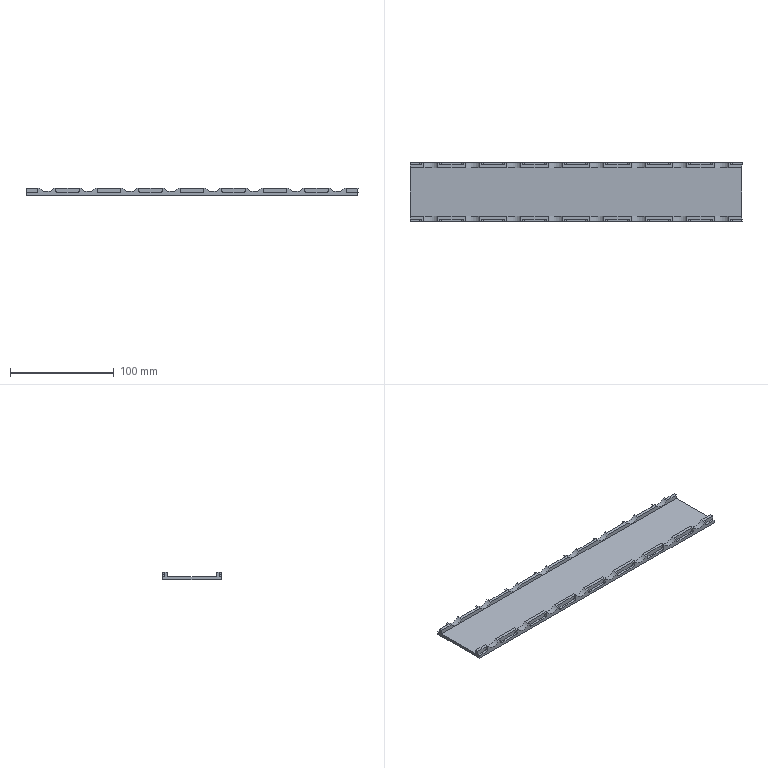NC program | Mastercam | posted with a generic post
Lines 1 to 1817 of 9376, first 1669 of 1817 lines:
%
:0001()
(MATERIAL - ALUMINUM MM - 2024)
(T1|8  RC |H1|D1|WEAR COMP|TOOL DIA. - 8.|XY STOCK TO LEAVE - .15|Z STOCK TO LEAVE - .5)
(T2|8 FI |H2)
(T3|4 RC |H3|D3|WEAR COMP|TOOL DIA. - 4.|XY STOCK TO LEAVE - .1|Z STOCK TO LEAVE - .1)
(T4|4 FI |H4|D4|WEAR COMP|TOOL DIA. - 4.)
(T5|2 BM/BNOS |H5)
N100 G21
N102 G0 G17 G40 G80 G90 G94 G98
N104 G0 G28 G91 Z0.
N106 G0 G28 X0. Y0.
(8  RC |TOOL - 1|DIA. OFF. - 1|LEN. - 1|TOOL DIA. - 8.)
N108 T1 M6
N110 G0 G54 G90 X172.55 Y.4 C0. B0. S6500 M3
N112 G43 H1 Z50.
N114 Z8.2
N116 G1 Z7.2 F2000.
N118 G41 D1 X164.55
N120 G3 X164.15 Y0. J-.4
N122 G1 Y-28.3 Z7.182
N124 X164.114 Y-28.842
N126 X164.009 Y-29.374 Z7.181
N128 X163.834 Y-29.888
N130 X163.594 Y-30.375
N132 X163.292 Y-30.826 Z7.18
N134 X162.934 Y-31.234
N136 X162.526 Y-31.592
N138 X162.075 Y-31.894 Z7.179
N140 X161.588 Y-32.134
N142 X161.074 Y-32.309
N144 X160.542 Y-32.414 Z7.178
N146 X160. Y-32.45
N148 X-160. Z6.972
N150 X-160.542 Y-32.414
N152 X-161.074 Y-32.309 Z6.971
N154 X-161.588 Y-32.134
N156 X-162.075 Y-31.894
N158 X-162.526 Y-31.592 Z6.97
N160 X-162.934 Y-31.234
N162 X-163.292 Y-30.826
N164 X-163.594 Y-30.375 Z6.969
N166 X-163.834 Y-29.888
N168 X-164.009 Y-29.374
N170 X-164.114 Y-28.842 Z6.968
N172 X-164.15 Y-28.3
N174 Y28.3 Z6.932
N176 X-164.114 Y28.842
N178 X-164.009 Y29.374 Z6.931
N180 X-163.834 Y29.888
N182 X-163.594 Y30.375
N184 X-163.292 Y30.826 Z6.93
N186 X-162.934 Y31.234
N188 X-162.526 Y31.592
N190 X-162.075 Y31.894 Z6.929
N192 X-161.588 Y32.134
N194 X-161.074 Y32.309
N196 X-160.542 Y32.414 Z6.928
N198 X-160. Y32.45
N200 X160. Z6.722
N202 X160.542 Y32.414
N204 X161.074 Y32.309 Z6.721
N206 X161.588 Y32.134
N208 X162.075 Y31.894
N210 X162.526 Y31.592 Z6.72
N212 X162.934 Y31.234
N214 X163.292 Y30.826
N216 X163.594 Y30.375 Z6.719
N218 X163.834 Y29.888
N220 X164.009 Y29.374
N222 X164.114 Y28.842 Z6.718
N224 X164.15 Y28.3
N226 Y0. Z6.7
N228 Y-28.3 Z6.682
N230 X164.114 Y-28.842
N232 X164.009 Y-29.374 Z6.681
N234 X163.834 Y-29.888
N236 X163.594 Y-30.375
N238 X163.292 Y-30.826 Z6.68
N240 X162.934 Y-31.234
N242 X162.526 Y-31.592
N244 X162.075 Y-31.894 Z6.679
N246 X161.588 Y-32.134
N248 X161.074 Y-32.309
N250 X160.542 Y-32.414 Z6.678
N252 X160. Y-32.45
N254 X-160. Z6.472
N256 X-160.542 Y-32.414
N258 X-161.074 Y-32.309 Z6.471
N260 X-161.588 Y-32.134
N262 X-162.075 Y-31.894
N264 X-162.526 Y-31.592 Z6.47
N266 X-162.934 Y-31.234
N268 X-163.292 Y-30.826
N270 X-163.594 Y-30.375 Z6.469
N272 X-163.834 Y-29.888
N274 X-164.009 Y-29.374
N276 X-164.114 Y-28.842 Z6.468
N278 X-164.15 Y-28.3
N280 Y28.3 Z6.432
N282 X-164.114 Y28.842
N284 X-164.009 Y29.374 Z6.431
N286 X-163.834 Y29.888
N288 X-163.594 Y30.375
N290 X-163.292 Y30.826 Z6.43
N292 X-162.934 Y31.234
N294 X-162.526 Y31.592
N296 X-162.075 Y31.894 Z6.429
N298 X-161.588 Y32.134
N300 X-161.074 Y32.309
N302 X-160.542 Y32.414 Z6.428
N304 X-160. Y32.45
N306 X160. Z6.222
N308 X160.542 Y32.414
N310 X161.074 Y32.309 Z6.221
N312 X161.588 Y32.134
N314 X162.075 Y31.894
N316 X162.526 Y31.592 Z6.22
N318 X162.934 Y31.234
N320 X163.292 Y30.826
N322 X163.594 Y30.375 Z6.219
N324 X163.834 Y29.888
N326 X164.009 Y29.374
N328 X164.114 Y28.842 Z6.218
N330 X164.15 Y28.3
N332 Y0. Z6.2
N334 Y-28.3 Z6.182
N336 X164.114 Y-28.842
N338 X164.009 Y-29.374 Z6.181
N340 X163.834 Y-29.888
N342 X163.594 Y-30.375
N344 X163.292 Y-30.826 Z6.18
N346 X162.934 Y-31.234
N348 X162.526 Y-31.592
N350 X162.075 Y-31.894 Z6.179
N352 X161.588 Y-32.134
N354 X161.074 Y-32.309
N356 X160.542 Y-32.414 Z6.178
N358 X160. Y-32.45
N360 X-160. Z5.972
N362 X-160.542 Y-32.414
N364 X-161.074 Y-32.309 Z5.971
N366 X-161.588 Y-32.134
N368 X-162.075 Y-31.894
N370 X-162.526 Y-31.592 Z5.97
N372 X-162.934 Y-31.234
N374 X-163.292 Y-30.826
N376 X-163.594 Y-30.375 Z5.969
N378 X-163.834 Y-29.888
N380 X-164.009 Y-29.374
N382 X-164.114 Y-28.842 Z5.968
N384 X-164.15 Y-28.3
N386 Y28.3 Z5.932
N388 X-164.114 Y28.842
N390 X-164.009 Y29.374 Z5.931
N392 X-163.834 Y29.888
N394 X-163.594 Y30.375
N396 X-163.292 Y30.826 Z5.93
N398 X-162.934 Y31.234
N400 X-162.526 Y31.592
N402 X-162.075 Y31.894 Z5.929
N404 X-161.588 Y32.134
N406 X-161.074 Y32.309
N408 X-160.542 Y32.414 Z5.928
N410 X-160. Y32.45
N412 X160. Z5.722
N414 X160.542 Y32.414
N416 X161.074 Y32.309 Z5.721
N418 X161.588 Y32.134
N420 X162.075 Y31.894
N422 X162.526 Y31.592 Z5.72
N424 X162.934 Y31.234
N426 X163.292 Y30.826
N428 X163.594 Y30.375 Z5.719
N430 X163.834 Y29.888
N432 X164.009 Y29.374
N434 X164.114 Y28.842 Z5.718
N436 X164.15 Y28.3
N438 Y0. Z5.7
N440 Y-28.3 Z5.682
N442 X164.114 Y-28.842
N444 X164.009 Y-29.374 Z5.681
N446 X163.834 Y-29.888
N448 X163.594 Y-30.375
N450 X163.292 Y-30.826 Z5.68
N452 X162.934 Y-31.234
N454 X162.526 Y-31.592
N456 X162.075 Y-31.894 Z5.679
N458 X161.588 Y-32.134
N460 X161.074 Y-32.309
N462 X160.542 Y-32.414 Z5.678
N464 X160. Y-32.45
N466 X-160. Z5.472
N468 X-160.542 Y-32.414
N470 X-161.074 Y-32.309 Z5.471
N472 X-161.588 Y-32.134
N474 X-162.075 Y-31.894
N476 X-162.526 Y-31.592 Z5.47
N478 X-162.934 Y-31.234
N480 X-163.292 Y-30.826
N482 X-163.594 Y-30.375 Z5.469
N484 X-163.834 Y-29.888
N486 X-164.009 Y-29.374
N488 X-164.114 Y-28.842 Z5.468
N490 X-164.15 Y-28.3
N492 Y28.3 Z5.432
N494 X-164.114 Y28.842
N496 X-164.009 Y29.374 Z5.431
N498 X-163.834 Y29.888
N500 X-163.594 Y30.375
N502 X-163.292 Y30.826 Z5.43
N504 X-162.934 Y31.234
N506 X-162.526 Y31.592
N508 X-162.075 Y31.894 Z5.429
N510 X-161.588 Y32.134
N512 X-161.074 Y32.309
N514 X-160.542 Y32.414 Z5.428
N516 X-160. Y32.45
N518 X160. Z5.222
N520 X160.542 Y32.414
N522 X161.074 Y32.309 Z5.221
N524 X161.588 Y32.134
N526 X162.075 Y31.894
N528 X162.526 Y31.592 Z5.22
N530 X162.934 Y31.234
N532 X163.292 Y30.826
N534 X163.594 Y30.375 Z5.219
N536 X163.834 Y29.888
N538 X164.009 Y29.374
N540 X164.114 Y28.842 Z5.218
N542 X164.15 Y28.3
N544 Y0. Z5.2
N546 Y-28.3 Z5.182
N548 X164.114 Y-28.842
N550 X164.009 Y-29.374 Z5.181
N552 X163.834 Y-29.888
N554 X163.594 Y-30.375
N556 X163.292 Y-30.826 Z5.18
N558 X162.934 Y-31.234
N560 X162.526 Y-31.592
N562 X162.075 Y-31.894 Z5.179
N564 X161.588 Y-32.134
N566 X161.074 Y-32.309
N568 X160.542 Y-32.414 Z5.178
N570 X160. Y-32.45
N572 X-160. Z4.972
N574 X-160.542 Y-32.414
N576 X-161.074 Y-32.309 Z4.971
N578 X-161.588 Y-32.134
N580 X-162.075 Y-31.894
N582 X-162.526 Y-31.592 Z4.97
N584 X-162.934 Y-31.234
N586 X-163.292 Y-30.826
N588 X-163.594 Y-30.375 Z4.969
N590 X-163.834 Y-29.888
N592 X-164.009 Y-29.374
N594 X-164.114 Y-28.842 Z4.968
N596 X-164.15 Y-28.3
N598 Y28.3 Z4.932
N600 X-164.114 Y28.842
N602 X-164.009 Y29.374 Z4.931
N604 X-163.834 Y29.888
N606 X-163.594 Y30.375
N608 X-163.292 Y30.826 Z4.93
N610 X-162.934 Y31.234
N612 X-162.526 Y31.592
N614 X-162.075 Y31.894 Z4.929
N616 X-161.588 Y32.134
N618 X-161.074 Y32.309
N620 X-160.542 Y32.414 Z4.928
N622 X-160. Y32.45
N624 X160. Z4.722
N626 X160.542 Y32.414
N628 X161.074 Y32.309 Z4.721
N630 X161.588 Y32.134
N632 X162.075 Y31.894
N634 X162.526 Y31.592 Z4.72
N636 X162.934 Y31.234
N638 X163.292 Y30.826
N640 X163.594 Y30.375 Z4.719
N642 X163.834 Y29.888
N644 X164.009 Y29.374
N646 X164.114 Y28.842 Z4.718
N648 X164.15 Y28.3
N650 Y0. Z4.7
N652 Y-28.3 Z4.682
N654 X164.114 Y-28.842
N656 X164.009 Y-29.374 Z4.681
N658 X163.834 Y-29.888
N660 X163.594 Y-30.375
N662 X163.292 Y-30.826 Z4.68
N664 X162.934 Y-31.234
N666 X162.526 Y-31.592
N668 X162.075 Y-31.894 Z4.679
N670 X161.588 Y-32.134
N672 X161.074 Y-32.309
N674 X160.542 Y-32.414 Z4.678
N676 X160. Y-32.45
N678 X-160. Z4.472
N680 X-160.542 Y-32.414
N682 X-161.074 Y-32.309 Z4.471
N684 X-161.588 Y-32.134
N686 X-162.075 Y-31.894
N688 X-162.526 Y-31.592 Z4.47
N690 X-162.934 Y-31.234
N692 X-163.292 Y-30.826
N694 X-163.594 Y-30.375 Z4.469
N696 X-163.834 Y-29.888
N698 X-164.009 Y-29.374
N700 X-164.114 Y-28.842 Z4.468
N702 X-164.15 Y-28.3
N704 Y28.3 Z4.432
N706 X-164.114 Y28.842
N708 X-164.009 Y29.374 Z4.431
N710 X-163.834 Y29.888
N712 X-163.594 Y30.375
N714 X-163.292 Y30.826 Z4.43
N716 X-162.934 Y31.234
N718 X-162.526 Y31.592
N720 X-162.075 Y31.894 Z4.429
N722 X-161.588 Y32.134
N724 X-161.074 Y32.309
N726 X-160.542 Y32.414 Z4.428
N728 X-160. Y32.45
N730 X160. Z4.222
N732 X160.542 Y32.414
N734 X161.074 Y32.309 Z4.221
N736 X161.588 Y32.134
N738 X162.075 Y31.894
N740 X162.526 Y31.592 Z4.22
N742 X162.934 Y31.234
N744 X163.292 Y30.826
N746 X163.594 Y30.375 Z4.219
N748 X163.834 Y29.888
N750 X164.009 Y29.374
N752 X164.114 Y28.842 Z4.218
N754 X164.15 Y28.3
N756 Y0. Z4.2
N758 Y-28.3 Z4.182
N760 X164.114 Y-28.842
N762 X164.009 Y-29.374 Z4.181
N764 X163.834 Y-29.888
N766 X163.594 Y-30.375
N768 X163.292 Y-30.826 Z4.18
N770 X162.934 Y-31.234
N772 X162.526 Y-31.592
N774 X162.075 Y-31.894 Z4.179
N776 X161.588 Y-32.134
N778 X161.074 Y-32.309
N780 X160.542 Y-32.414 Z4.178
N782 X160. Y-32.45
N784 X-160. Z3.972
N786 X-160.542 Y-32.414
N788 X-161.074 Y-32.309 Z3.971
N790 X-161.588 Y-32.134
N792 X-162.075 Y-31.894
N794 X-162.526 Y-31.592 Z3.97
N796 X-162.934 Y-31.234
N798 X-163.292 Y-30.826
N800 X-163.594 Y-30.375 Z3.969
N802 X-163.834 Y-29.888
N804 X-164.009 Y-29.374
N806 X-164.114 Y-28.842 Z3.968
N808 X-164.15 Y-28.3
N810 Y28.3 Z3.932
N812 X-164.114 Y28.842
N814 X-164.009 Y29.374 Z3.931
N816 X-163.834 Y29.888
N818 X-163.594 Y30.375
N820 X-163.292 Y30.826 Z3.93
N822 X-162.934 Y31.234
N824 X-162.526 Y31.592
N826 X-162.075 Y31.894 Z3.929
N828 X-161.588 Y32.134
N830 X-161.074 Y32.309
N832 X-160.542 Y32.414 Z3.928
N834 X-160. Y32.45
N836 X160. Z3.722
N838 X160.542 Y32.414
N840 X161.074 Y32.309 Z3.721
N842 X161.588 Y32.134
N844 X162.075 Y31.894
N846 X162.526 Y31.592 Z3.72
N848 X162.934 Y31.234
N850 X163.292 Y30.826
N852 X163.594 Y30.375 Z3.719
N854 X163.834 Y29.888
N856 X164.009 Y29.374
N858 X164.114 Y28.842 Z3.718
N860 X164.15 Y28.3
N862 Y0. Z3.7
N864 Y-28.3 Z3.682
N866 X164.114 Y-28.842
N868 X164.009 Y-29.374 Z3.681
N870 X163.834 Y-29.888
N872 X163.594 Y-30.375
N874 X163.292 Y-30.826 Z3.68
N876 X162.934 Y-31.234
N878 X162.526 Y-31.592
N880 X162.075 Y-31.894 Z3.679
N882 X161.588 Y-32.134
N884 X161.074 Y-32.309
N886 X160.542 Y-32.414 Z3.678
N888 X160. Y-32.45
N890 X-160. Z3.472
N892 X-160.542 Y-32.414
N894 X-161.074 Y-32.309 Z3.471
N896 X-161.588 Y-32.134
N898 X-162.075 Y-31.894
N900 X-162.526 Y-31.592 Z3.47
N902 X-162.934 Y-31.234
N904 X-163.292 Y-30.826
N906 X-163.594 Y-30.375 Z3.469
N908 X-163.834 Y-29.888
N910 X-164.009 Y-29.374
N912 X-164.114 Y-28.842 Z3.468
N914 X-164.15 Y-28.3
N916 Y28.3 Z3.432
N918 X-164.114 Y28.842
N920 X-164.009 Y29.374 Z3.431
N922 X-163.834 Y29.888
N924 X-163.594 Y30.375
N926 X-163.292 Y30.826 Z3.43
N928 X-162.934 Y31.234
N930 X-162.526 Y31.592
N932 X-162.075 Y31.894 Z3.429
N934 X-161.588 Y32.134
N936 X-161.074 Y32.309
N938 X-160.542 Y32.414 Z3.428
N940 X-160. Y32.45
N942 X160. Z3.222
N944 X160.542 Y32.414
N946 X161.074 Y32.309 Z3.221
N948 X161.588 Y32.134
N950 X162.075 Y31.894
N952 X162.526 Y31.592 Z3.22
N954 X162.934 Y31.234
N956 X163.292 Y30.826
N958 X163.594 Y30.375 Z3.219
N960 X163.834 Y29.888
N962 X164.009 Y29.374
N964 X164.114 Y28.842 Z3.218
N966 X164.15 Y28.3
N968 Y0. Z3.2
N970 Y-28.3 Z3.182
N972 X164.114 Y-28.842
N974 X164.009 Y-29.374 Z3.181
N976 X163.834 Y-29.888
N978 X163.594 Y-30.375
N980 X163.292 Y-30.826 Z3.18
N982 X162.934 Y-31.234
N984 X162.526 Y-31.592
N986 X162.075 Y-31.894 Z3.179
N988 X161.588 Y-32.134
N990 X161.074 Y-32.309
N992 X160.542 Y-32.414 Z3.178
N994 X160. Y-32.45
N996 X-160. Z2.972
N998 X-160.542 Y-32.414
N1000 X-161.074 Y-32.309 Z2.971
N1002 X-161.588 Y-32.134
N1004 X-162.075 Y-31.894
N1006 X-162.526 Y-31.592 Z2.97
N1008 X-162.934 Y-31.234
N1010 X-163.292 Y-30.826
N1012 X-163.594 Y-30.375 Z2.969
N1014 X-163.834 Y-29.888
N1016 X-164.009 Y-29.374
N1018 X-164.114 Y-28.842 Z2.968
N1020 X-164.15 Y-28.3
N1022 Y28.3 Z2.932
N1024 X-164.114 Y28.842
N1026 X-164.009 Y29.374 Z2.931
N1028 X-163.834 Y29.888
N1030 X-163.594 Y30.375
N1032 X-163.292 Y30.826 Z2.93
N1034 X-162.934 Y31.234
N1036 X-162.526 Y31.592
N1038 X-162.075 Y31.894 Z2.929
N1040 X-161.588 Y32.134
N1042 X-161.074 Y32.309
N1044 X-160.542 Y32.414 Z2.928
N1046 X-160. Y32.45
N1048 X160. Z2.722
N1050 X160.542 Y32.414
N1052 X161.074 Y32.309 Z2.721
N1054 X161.588 Y32.134
N1056 X162.075 Y31.894
N1058 X162.526 Y31.592 Z2.72
N1060 X162.934 Y31.234
N1062 X163.292 Y30.826
N1064 X163.594 Y30.375 Z2.719
N1066 X163.834 Y29.888
N1068 X164.009 Y29.374
N1070 X164.114 Y28.842 Z2.718
N1072 X164.15 Y28.3
N1074 Y0. Z2.7
N1076 Y-28.3 Z2.682
N1078 X164.114 Y-28.842
N1080 X164.009 Y-29.374 Z2.681
N1082 X163.834 Y-29.888
N1084 X163.594 Y-30.375
N1086 X163.292 Y-30.826 Z2.68
N1088 X162.934 Y-31.234
N1090 X162.526 Y-31.592
N1092 X162.075 Y-31.894 Z2.679
N1094 X161.588 Y-32.134
N1096 X161.074 Y-32.309
N1098 X160.542 Y-32.414 Z2.678
N1100 X160. Y-32.45
N1102 X-160. Z2.472
N1104 X-160.542 Y-32.414
N1106 X-161.074 Y-32.309 Z2.471
N1108 X-161.588 Y-32.134
N1110 X-162.075 Y-31.894
N1112 X-162.526 Y-31.592 Z2.47
N1114 X-162.934 Y-31.234
N1116 X-163.292 Y-30.826
N1118 X-163.594 Y-30.375 Z2.469
N1120 X-163.834 Y-29.888
N1122 X-164.009 Y-29.374
N1124 X-164.114 Y-28.842 Z2.468
N1126 X-164.15 Y-28.3
N1128 Y28.3 Z2.432
N1130 X-164.114 Y28.842
N1132 X-164.009 Y29.374 Z2.431
N1134 X-163.834 Y29.888
N1136 X-163.594 Y30.375
N1138 X-163.292 Y30.826 Z2.43
N1140 X-162.934 Y31.234
N1142 X-162.526 Y31.592
N1144 X-162.075 Y31.894 Z2.429
N1146 X-161.588 Y32.134
N1148 X-161.074 Y32.309
N1150 X-160.542 Y32.414 Z2.428
N1152 X-160. Y32.45
N1154 X160. Z2.222
N1156 X160.542 Y32.414
N1158 X161.074 Y32.309 Z2.221
N1160 X161.588 Y32.134
N1162 X162.075 Y31.894
N1164 X162.526 Y31.592 Z2.22
N1166 X162.934 Y31.234
N1168 X163.292 Y30.826
N1170 X163.594 Y30.375 Z2.219
N1172 X163.834 Y29.888
N1174 X164.009 Y29.374
N1176 X164.114 Y28.842 Z2.218
N1178 X164.15 Y28.3
N1180 Y0. Z2.2
N1182 Y-28.3 Z2.182
N1184 X164.114 Y-28.842
N1186 X164.009 Y-29.374 Z2.181
N1188 X163.834 Y-29.888
N1190 X163.594 Y-30.375
N1192 X163.292 Y-30.826 Z2.18
N1194 X162.934 Y-31.234
N1196 X162.526 Y-31.592
N1198 X162.075 Y-31.894 Z2.179
N1200 X161.588 Y-32.134
N1202 X161.074 Y-32.309
N1204 X160.542 Y-32.414 Z2.178
N1206 X160. Y-32.45
N1208 X-160. Z1.972
N1210 X-160.542 Y-32.414
N1212 X-161.074 Y-32.309 Z1.971
N1214 X-161.588 Y-32.134
N1216 X-162.075 Y-31.894
N1218 X-162.526 Y-31.592 Z1.97
N1220 X-162.934 Y-31.234
N1222 X-163.292 Y-30.826
N1224 X-163.594 Y-30.375 Z1.969
N1226 X-163.834 Y-29.888
N1228 X-164.009 Y-29.374
N1230 X-164.114 Y-28.842 Z1.968
N1232 X-164.15 Y-28.3
N1234 Y28.3 Z1.932
N1236 X-164.114 Y28.842
N1238 X-164.009 Y29.374 Z1.931
N1240 X-163.834 Y29.888
N1242 X-163.594 Y30.375
N1244 X-163.292 Y30.826 Z1.93
N1246 X-162.934 Y31.234
N1248 X-162.526 Y31.592
N1250 X-162.075 Y31.894 Z1.929
N1252 X-161.588 Y32.134
N1254 X-161.074 Y32.309
N1256 X-160.542 Y32.414 Z1.928
N1258 X-160. Y32.45
N1260 X160. Z1.722
N1262 X160.542 Y32.414
N1264 X161.074 Y32.309 Z1.721
N1266 X161.588 Y32.134
N1268 X162.075 Y31.894
N1270 X162.526 Y31.592 Z1.72
N1272 X162.934 Y31.234
N1274 X163.292 Y30.826
N1276 X163.594 Y30.375 Z1.719
N1278 X163.834 Y29.888
N1280 X164.009 Y29.374
N1282 X164.114 Y28.842 Z1.718
N1284 X164.15 Y28.3
N1286 Y0. Z1.7
N1288 Y-28.3 Z1.682
N1290 X164.114 Y-28.842
N1292 X164.009 Y-29.374 Z1.681
N1294 X163.834 Y-29.888
N1296 X163.594 Y-30.375
N1298 X163.292 Y-30.826 Z1.68
N1300 X162.934 Y-31.234
N1302 X162.526 Y-31.592
N1304 X162.075 Y-31.894 Z1.679
N1306 X161.588 Y-32.134
N1308 X161.074 Y-32.309
N1310 X160.542 Y-32.414 Z1.678
N1312 X160. Y-32.45
N1314 X-160. Z1.472
N1316 X-160.542 Y-32.414
N1318 X-161.074 Y-32.309 Z1.471
N1320 X-161.588 Y-32.134
N1322 X-162.075 Y-31.894
N1324 X-162.526 Y-31.592 Z1.47
N1326 X-162.934 Y-31.234
N1328 X-163.292 Y-30.826
N1330 X-163.594 Y-30.375 Z1.469
N1332 X-163.834 Y-29.888
N1334 X-164.009 Y-29.374
N1336 X-164.114 Y-28.842 Z1.468
N1338 X-164.15 Y-28.3
N1340 Y28.3 Z1.432
N1342 X-164.114 Y28.842
N1344 X-164.009 Y29.374 Z1.431
N1346 X-163.834 Y29.888
N1348 X-163.594 Y30.375
N1350 X-163.292 Y30.826 Z1.43
N1352 X-162.934 Y31.234
N1354 X-162.526 Y31.592
N1356 X-162.075 Y31.894 Z1.429
N1358 X-161.588 Y32.134
N1360 X-161.074 Y32.309
N1362 X-160.542 Y32.414 Z1.428
N1364 X-160. Y32.45
N1366 X160. Z1.222
N1368 X160.542 Y32.414
N1370 X161.074 Y32.309 Z1.221
N1372 X161.588 Y32.134
N1374 X162.075 Y31.894
N1376 X162.526 Y31.592 Z1.22
N1378 X162.934 Y31.234
N1380 X163.292 Y30.826
N1382 X163.594 Y30.375 Z1.219
N1384 X163.834 Y29.888
N1386 X164.009 Y29.374
N1388 X164.114 Y28.842 Z1.218
N1390 X164.15 Y28.3
N1392 Y0. Z1.2
N1394 Y-28.3 Z1.182
N1396 X164.114 Y-28.842
N1398 X164.009 Y-29.374 Z1.181
N1400 X163.834 Y-29.888
N1402 X163.594 Y-30.375
N1404 X163.292 Y-30.826 Z1.18
N1406 X162.934 Y-31.234
N1408 X162.526 Y-31.592
N1410 X162.075 Y-31.894 Z1.179
N1412 X161.588 Y-32.134
N1414 X161.074 Y-32.309
N1416 X160.542 Y-32.414 Z1.178
N1418 X160. Y-32.45
N1420 X-160. Z.972
N1422 X-160.542 Y-32.414
N1424 X-161.074 Y-32.309 Z.971
N1426 X-161.588 Y-32.134
N1428 X-162.075 Y-31.894
N1430 X-162.526 Y-31.592 Z.97
N1432 X-162.934 Y-31.234
N1434 X-163.292 Y-30.826
N1436 X-163.594 Y-30.375 Z.969
N1438 X-163.834 Y-29.888
N1440 X-164.009 Y-29.374
N1442 X-164.114 Y-28.842 Z.968
N1444 X-164.15 Y-28.3
N1446 Y28.3 Z.932
N1448 X-164.114 Y28.842
N1450 X-164.009 Y29.374 Z.931
N1452 X-163.834 Y29.888
N1454 X-163.594 Y30.375
N1456 X-163.292 Y30.826 Z.93
N1458 X-162.934 Y31.234
N1460 X-162.526 Y31.592
N1462 X-162.075 Y31.894 Z.929
N1464 X-161.588 Y32.134
N1466 X-161.074 Y32.309
N1468 X-160.542 Y32.414 Z.928
N1470 X-160. Y32.45
N1472 X160. Z.722
N1474 X160.542 Y32.414
N1476 X161.074 Y32.309 Z.721
N1478 X161.588 Y32.134
N1480 X162.075 Y31.894
N1482 X162.526 Y31.592 Z.72
N1484 X162.934 Y31.234
N1486 X163.292 Y30.826
N1488 X163.594 Y30.375 Z.719
N1490 X163.834 Y29.888
N1492 X164.009 Y29.374
N1494 X164.114 Y28.842 Z.718
N1496 X164.15 Y28.3
N1498 Y0. Z.7
N1500 Y-28.3 Z.682
N1502 X164.114 Y-28.842
N1504 X164.009 Y-29.374 Z.681
N1506 X163.834 Y-29.888
N1508 X163.594 Y-30.375
N1510 X163.292 Y-30.826 Z.68
N1512 X162.934 Y-31.234
N1514 X162.526 Y-31.592
N1516 X162.075 Y-31.894 Z.679
N1518 X161.588 Y-32.134
N1520 X161.074 Y-32.309
N1522 X160.542 Y-32.414 Z.678
N1524 X160. Y-32.45
N1526 X-116.891 Z.5
N1528 X-160.
N1530 G2 X-164.15 Y-28.3 J4.15
N1532 G1 Y28.3
N1534 G2 X-160. Y32.45 I4.15
N1536 G1 X160.
N1538 G2 X164.15 Y28.3 J-4.15
N1540 G1 Y0.
N1542 Y-28.3
N1544 G2 X160. Y-32.45 I-4.15
N1546 G1 X-117.391
N1548 G3 X-117.791 Y-32.85 J-.4
N1550 G1 G40 Y-40.85
N1552 G0 Z50.
N1554 X-163.366 Y-2.865
N1556 Z10.
N1558 G1 Z8.2
N1560 X-156.85 Z7.859
N1562 X-164.85 Z7.439
N1564 X-156.85 Z7.02
N1566 X-150.35 Y-3.15
N1568 X150.35
N1570 Y1.85
N1572 X-150.35
N1574 Y-3.15
N1576 X-154.35 Y-7.15
N1578 X154.35
N1580 Y6.35
N1582 X-154.35
N1584 Y-7.15
N1586 X-158.35 Y-11.15
N1588 X158.35
N1590 Y10.85
N1592 X-158.35
N1594 Y-11.15
N1596 X-162.35 Y-15.15
N1598 X162.35
N1600 Y15.35
N1602 X-162.35
N1604 Y-15.15
N1606 X-165.85 Y-19.15
N1608 X165.85
N1610 Y19.15
N1612 X-165.85
N1614 Y-19.15
N1616 G0 Z50.
N1618 X-163.366 Y-2.865
N1620 Z9.02
N1622 G1 Z7.22
N1624 X-156.85 Z6.879
N1626 X-164.85 Z6.459
N1628 X-156.85 Z6.04
N1630 X-150.35 Y-3.15
N1632 X150.35
N1634 Y1.85
N1636 X-150.35
N1638 Y-3.15
N1640 X-154.35 Y-7.15
N1642 X154.35
N1644 Y6.35
N1646 X-154.35
N1648 Y-7.15
N1650 X-158.35 Y-11.15
N1652 X158.35
N1654 Y10.85
N1656 X-158.35
N1658 Y-11.15
N1660 X-162.35 Y-15.15
N1662 X162.35
N1664 Y15.35
N1666 X-162.35
N1668 Y-15.15
N1670 X-165.85 Y-19.15
N1672 X165.85
N1674 Y19.15
N1676 X-165.85
N1678 Y-19.15
N1680 G0 Z50.
N1682 X-163.366 Y-2.865
N1684 Z8.04
N1686 G1 Z6.24
N1688 X-156.85 Z5.899
N1690 X-164.85 Z5.479
N1692 X-156.85 Z5.06
N1694 X-150.35 Y-3.15
N1696 X150.35
N1698 Y1.85
N1700 X-150.35
N1702 Y-3.15
N1704 X-154.35 Y-7.15
N1706 X154.35
N1708 Y6.35
N1710 X-154.35
N1712 Y-7.15
N1714 X-158.35 Y-11.15
N1716 X158.35
N1718 Y10.85
N1720 X-158.35
N1722 Y-11.15
N1724 X-162.35 Y-15.15
N1726 X162.35
N1728 Y15.35
N1730 X-162.35
N1732 Y-15.15
N1734 X-165.85 Y-19.15
N1736 X165.85
N1738 Y19.15
N1740 X-165.85
N1742 Y-19.15
N1744 G0 Z50.
N1746 X-163.366 Y-2.865
N1748 Z7.06
N1750 G1 Z5.26
N1752 X-156.85 Z4.919
N1754 X-164.85 Z4.499
N1756 X-156.85 Z4.08
N1758 X-150.35 Y-3.15
N1760 X150.35
N1762 Y1.85
N1764 X-150.35
N1766 Y-3.15
N1768 X-154.35 Y-7.15
N1770 X154.35
N1772 Y6.35
N1774 X-154.35
N1776 Y-7.15
N1778 X-158.35 Y-11.15
N1780 X158.35
N1782 Y10.85
N1784 X-158.35
N1786 Y-11.15
N1788 X-162.35 Y-15.15
N1790 X162.35
N1792 Y15.35
N1794 X-162.35
N1796 Y-15.15
N1798 X-165.85 Y-19.15
N1800 X165.85
N1802 Y19.15
N1804 X-165.85
N1806 Y-19.15
N1808 G0 Z50.
N1810 X-163.366 Y-2.865
N1812 Z6.08
N1814 G1 Z4.28
N1816 X-156.85 Z3.939
N1818 X-164.85 Z3.519
N1820 X-156.85 Z3.1
N1822 X-150.35 Y-3.15
N1824 X150.35
N1826 Y1.85
N1828 X-150.35
N1830 Y-3.15
N1832 X-154.35 Y-7.15
N1834 X154.35
N1836 Y6.35
N1838 X-154.35
N1840 Y-7.15
N1842 X-158.35 Y-11.15
N1844 X158.35
N1846 Y10.85
N1848 X-158.35
N1850 Y-11.15
N1852 X-162.35 Y-15.15
N1854 X162.35
N1856 Y15.35
N1858 X-162.35
N1860 Y-15.15
N1862 X-165.85 Y-19.15
N1864 X165.85
N1866 Y19.15
N1868 X-165.85
N1870 Y-19.15
N1872 G0 Z50.
N1874 S5000 M3
N1876 X-168. Y26.3
N1878 Z8.1
N1880 G1 Z7.1
N1882 G41 D1 X-160. F600.
N1884 X160.
N1886 G40 X168.
N1888 G0 Z50.
N1890 X167.987 Y-27.735
N1892 Z8.1
N1894 G1 Z7.1 F2000.
N1896 G41 D1 X159.987 Y-27.7 F600.
N1898 X-160.013 Y-26.3
N1900 G40 X-168.013 Y-26.265
N1902 G0 Z50.
N1904 M5
N1906 G0 G28 G91 Z0.
N1908 G28
N1910 M01
N1912 G0 G17 G40 G80 G90 G94 G98
N1914 G0 G28 G91 Z0.
(8 FI |TOOL - 2|DIA. OFF. - 2|LEN. - 2|TOOL DIA. - 8.)
N1916 T2 M6
N1918 G0 G54 G90 X-160.222 Y-2.889 C0. B0. S6500 M3
N1920 G43 H2 Z50.
N1922 Z10.
N1924 G1 Z8.2 F2000.
N1926 X-157. Z8.031
N1928 X-165. Z7.612
N1930 X-157. Z7.193
N1932 X-165. Z6.773
N1934 X-157. Z6.354
N1936 X-165. Z5.935
N1938 X-157. Z5.516
N1940 X-165. Z5.096
N1942 X-157. Z4.677
N1944 X-165. Z4.258
N1946 X-157. Z3.839
N1948 X-165. Z3.419
N1950 X-157. Z3.
N1952 X-150.5 Y-3.8 F1000.
N1954 X150.5
N1956 Y2.2
N1958 X-150.5
N1960 Y-3.8
N1962 X-154.5 Y-7.8
N1964 X154.5
N1966 Y6.7
N1968 X-154.5
N1970 Y-7.8
N1972 X-158.5 Y-11.8
N1974 X158.5
N1976 Y11.2
N1978 X-158.5
N1980 Y-11.8
N1982 X-162.5 Y-15.8
N1984 X162.5
N1986 Y15.7
N1988 X-162.5
N1990 Y-15.8
N1992 X-166. Y-19.3
N1994 X166.
N1996 Y19.3
N1998 X-166.
N2000 Y-19.3
N2002 G0 Z50.
N2004 M5
N2006 G0 G28 G91 Z0.
N2008 G28
N2010 M01
N2012 G0 G17 G40 G80 G90 G94 G98
N2014 G0 G28 G91 Z0.
(8  RC |TOOL - 1|DIA. OFF. - 1|LEN. - 1|TOOL DIA. - 8.)
N2016 T1 M6
N2018 G0 G54 G90 X-168. Y26.3 C0. B0. S5000 M3
N2020 G43 H1 Z50.
N2022 Z8.
N2024 G1 Z7. F2000.
N2026 G41 D1 X-160. F600.
N2028 X160.
N2030 G40 X168.
N2032 G0 Z50.
N2034 X167.987 Y-27.735
N2036 Z8.
N2038 G1 Z7. F2000.
N2040 G41 D1 X159.987 Y-27.7 F600.
N2042 X-160.013 Y-26.3
N2044 G40 X-168.013 Y-26.265
N2046 G0 Z50.
N2048 Z78.3
N2050 X15.771 Y149.046
N2052 B-90.
N2054 Z33.3
N2056 G1 Z31.8 F2000.
N2058 G41 D1 X9.707 Y143.828 F1000.
N2060 G3 X7.951 Y140. I3.293 J-3.828
N2062 X9.707 Y136.172 I5.049
N2064 G1 G40 X15.771 Y130.954
N2066 Z31.3 F2000.
N2068 G42 D1 X9.707 Y136.172 F1000.
N2070 G2 X7.951 Y140. I3.293 J3.828
N2072 X9.707 Y143.828 I5.049
N2074 G1 G40 X15.771 Y149.046
N2076 Z30.8 F2000.
N2078 G41 D1 X9.707 Y143.828 F1000.
N2080 G3 X7.951 Y140. I3.293 J-3.828
N2082 X9.707 Y136.172 I5.049
N2084 G1 G40 X15.771 Y130.954
N2086 Z30.3 F2000.
N2088 G42 D1 X9.707 Y136.172 F1000.
N2090 G2 X7.951 Y140. I3.293 J3.828
N2092 X9.707 Y143.828 I5.049
N2094 G1 G40 X15.771 Y149.046
N2096 Z29.8 F2000.
N2098 G41 D1 X9.707 Y143.828 F1000.
N2100 G3 X7.951 Y140. I3.293 J-3.828
N2102 X9.707 Y136.172 I5.049
N2104 G1 G40 X15.771 Y130.954
N2106 Z29.3 F2000.
N2108 G42 D1 X9.707 Y136.172 F1000.
N2110 G2 X7.951 Y140. I3.293 J3.828
N2112 X9.707 Y143.828 I5.049
N2114 G1 G40 X15.771 Y149.046
N2116 Z28.8 F2000.
N2118 G41 D1 X9.707 Y143.828 F1000.
N2120 G3 X7.951 Y140. I3.293 J-3.828
N2122 X9.707 Y136.172 I5.049
N2124 G1 G40 X15.771 Y130.954
N2126 Z28.3 F2000.
N2128 G42 D1 X9.707 Y136.172 F1000.
N2130 G2 X7.951 Y140. I3.293 J3.828
N2132 X9.707 Y143.828 I5.049
N2134 G1 G40 X15.771 Y149.046
N2136 Z27.8 F2000.
N2138 G41 D1 X9.707 Y143.828 F1000.
N2140 G3 X7.951 Y140. I3.293 J-3.828
N2142 X9.707 Y136.172 I5.049
N2144 G1 G40 X15.771 Y130.954
N2146 Z27.3 F2000.
N2148 G42 D1 X9.707 Y136.172 F1000.
N2150 G2 X7.951 Y140. I3.293 J3.828
N2152 X9.707 Y143.828 I5.049
N2154 G1 G40 X15.771 Y149.046
N2156 Z26.8 F2000.
N2158 G41 D1 X9.707 Y143.828 F1000.
N2160 G3 X7.951 Y140. I3.293 J-3.828
N2162 X9.707 Y136.172 I5.049
N2164 G1 G40 X15.771 Y130.954
N2166 Z26.3 F2000.
N2168 G42 D1 X9.707 Y136.172 F1000.
N2170 G2 X7.951 Y140. I3.293 J3.828
N2172 X9.707 Y143.828 I5.049
N2174 G1 G40 X15.771 Y149.046
N2176 Z25.8 F2000.
N2178 G41 D1 X9.707 Y143.828 F1000.
N2180 G3 X7.951 Y140. I3.293 J-3.828
N2182 X9.707 Y136.172 I5.049
N2184 G1 G40 X15.771 Y130.954
N2186 Z25.3 F2000.
N2188 G42 D1 X9.707 Y136.172 F1000.
N2190 G2 X7.951 Y140. I3.293 J3.828
N2192 X9.707 Y143.828 I5.049
N2194 G1 G40 X15.771 Y149.046
N2196 Z24.8 F2000.
N2198 G41 D1 X9.707 Y143.828 F1000.
N2200 G3 X7.951 Y140. I3.293 J-3.828
N2202 X9.707 Y136.172 I5.049
N2204 G1 G40 X15.771 Y130.954
N2206 Z24.3 F2000.
N2208 G42 D1 X9.707 Y136.172 F1000.
N2210 G2 X7.951 Y140. I3.293 J3.828
N2212 X9.707 Y143.828 I5.049
N2214 G1 G40 X15.771 Y149.046
N2216 Z23.8 F2000.
N2218 G41 D1 X9.707 Y143.828 F1000.
N2220 G3 X7.951 Y140. I3.293 J-3.828
N2222 X9.707 Y136.172 I5.049
N2224 G1 G40 X15.771 Y130.954
N2226 Z23.3 F2000.
N2228 G42 D1 X9.707 Y136.172 F1000.
N2230 G2 X7.951 Y140. I3.293 J3.828
N2232 X9.707 Y143.828 I5.049
N2234 G1 G40 X15.771 Y149.046
N2236 Z22.8 F2000.
N2238 G41 D1 X9.707 Y143.828 F1000.
N2240 G3 X7.951 Y140. I3.293 J-3.828
N2242 X9.707 Y136.172 I5.049
N2244 G1 G40 X15.771 Y130.954
N2246 Z22.3 F2000.
N2248 G42 D1 X9.707 Y136.172 F1000.
N2250 G2 X7.951 Y140. I3.293 J3.828
N2252 X9.707 Y143.828 I5.049
N2254 G1 G40 X15.771 Y149.046
N2256 G0 Z78.3
N2258 Y109.046
N2260 Z33.3
N2262 G1 Z31.8 F2000.
N2264 G41 D1 X9.707 Y103.828 F1000.
N2266 G3 X7.951 Y100. I3.293 J-3.828
N2268 X9.707 Y96.172 I5.049
N2270 G1 G40 X15.771 Y90.954
N2272 Z31.3 F2000.
N2274 G42 D1 X9.707 Y96.172 F1000.
N2276 G2 X7.951 Y100. I3.293 J3.828
N2278 X9.707 Y103.828 I5.049
N2280 G1 G40 X15.771 Y109.046
N2282 Z30.8 F2000.
N2284 G41 D1 X9.707 Y103.828 F1000.
N2286 G3 X7.951 Y100. I3.293 J-3.828
N2288 X9.707 Y96.172 I5.049
N2290 G1 G40 X15.771 Y90.954
N2292 Z30.3 F2000.
N2294 G42 D1 X9.707 Y96.172 F1000.
N2296 G2 X7.951 Y100. I3.293 J3.828
N2298 X9.707 Y103.828 I5.049
N2300 G1 G40 X15.771 Y109.046
N2302 Z29.8 F2000.
N2304 G41 D1 X9.707 Y103.828 F1000.
N2306 G3 X7.951 Y100. I3.293 J-3.828
N2308 X9.707 Y96.172 I5.049
N2310 G1 G40 X15.771 Y90.954
N2312 Z29.3 F2000.
N2314 G42 D1 X9.707 Y96.172 F1000.
N2316 G2 X7.951 Y100. I3.293 J3.828
N2318 X9.707 Y103.828 I5.049
N2320 G1 G40 X15.771 Y109.046
N2322 Z28.8 F2000.
N2324 G41 D1 X9.707 Y103.828 F1000.
N2326 G3 X7.951 Y100. I3.293 J-3.828
N2328 X9.707 Y96.172 I5.049
N2330 G1 G40 X15.771 Y90.954
N2332 Z28.3 F2000.
N2334 G42 D1 X9.707 Y96.172 F1000.
N2336 G2 X7.951 Y100. I3.293 J3.828
N2338 X9.707 Y103.828 I5.049
N2340 G1 G40 X15.771 Y109.046
N2342 Z27.8 F2000.
N2344 G41 D1 X9.707 Y103.828 F1000.
N2346 G3 X7.951 Y100. I3.293 J-3.828
N2348 X9.707 Y96.172 I5.049
N2350 G1 G40 X15.771 Y90.954
N2352 Z27.3 F2000.
N2354 G42 D1 X9.707 Y96.172 F1000.
N2356 G2 X7.951 Y100. I3.293 J3.828
N2358 X9.707 Y103.828 I5.049
N2360 G1 G40 X15.771 Y109.046
N2362 Z26.8 F2000.
N2364 G41 D1 X9.707 Y103.828 F1000.
N2366 G3 X7.951 Y100. I3.293 J-3.828
N2368 X9.707 Y96.172 I5.049
N2370 G1 G40 X15.771 Y90.954
N2372 Z26.3 F2000.
N2374 G42 D1 X9.707 Y96.172 F1000.
N2376 G2 X7.951 Y100. I3.293 J3.828
N2378 X9.707 Y103.828 I5.049
N2380 G1 G40 X15.771 Y109.046
N2382 Z25.8 F2000.
N2384 G41 D1 X9.707 Y103.828 F1000.
N2386 G3 X7.951 Y100. I3.293 J-3.828
N2388 X9.707 Y96.172 I5.049
N2390 G1 G40 X15.771 Y90.954
N2392 Z25.3 F2000.
N2394 G42 D1 X9.707 Y96.172 F1000.
N2396 G2 X7.951 Y100. I3.293 J3.828
N2398 X9.707 Y103.828 I5.049
N2400 G1 G40 X15.771 Y109.046
N2402 Z24.8 F2000.
N2404 G41 D1 X9.707 Y103.828 F1000.
N2406 G3 X7.951 Y100. I3.293 J-3.828
N2408 X9.707 Y96.172 I5.049
N2410 G1 G40 X15.771 Y90.954
N2412 Z24.3 F2000.
N2414 G42 D1 X9.707 Y96.172 F1000.
N2416 G2 X7.951 Y100. I3.293 J3.828
N2418 X9.707 Y103.828 I5.049
N2420 G1 G40 X15.771 Y109.046
N2422 Z23.8 F2000.
N2424 G41 D1 X9.707 Y103.828 F1000.
N2426 G3 X7.951 Y100. I3.293 J-3.828
N2428 X9.707 Y96.172 I5.049
N2430 G1 G40 X15.771 Y90.954
N2432 Z23.3 F2000.
N2434 G42 D1 X9.707 Y96.172 F1000.
N2436 G2 X7.951 Y100. I3.293 J3.828
N2438 X9.707 Y103.828 I5.049
N2440 G1 G40 X15.771 Y109.046
N2442 Z22.8 F2000.
N2444 G41 D1 X9.707 Y103.828 F1000.
N2446 G3 X7.951 Y100. I3.293 J-3.828
N2448 X9.707 Y96.172 I5.049
N2450 G1 G40 X15.771 Y90.954
N2452 Z22.3 F2000.
N2454 G42 D1 X9.707 Y96.172 F1000.
N2456 G2 X7.951 Y100. I3.293 J3.828
N2458 X9.707 Y103.828 I5.049
N2460 G1 G40 X15.771 Y109.046
N2462 G0 Z78.3
N2464 Y69.046
N2466 Z33.3
N2468 G1 Z31.8 F2000.
N2470 G41 D1 X9.707 Y63.828 F1000.
N2472 G3 X7.951 Y60. I3.293 J-3.828
N2474 X9.707 Y56.172 I5.049
N2476 G1 G40 X15.771 Y50.954
N2478 Z31.3 F2000.
N2480 G42 D1 X9.707 Y56.172 F1000.
N2482 G2 X7.951 Y60. I3.293 J3.828
N2484 X9.707 Y63.828 I5.049
N2486 G1 G40 X15.771 Y69.046
N2488 Z30.8 F2000.
N2490 G41 D1 X9.707 Y63.828 F1000.
N2492 G3 X7.951 Y60. I3.293 J-3.828
N2494 X9.707 Y56.172 I5.049
N2496 G1 G40 X15.771 Y50.954
N2498 Z30.3 F2000.
N2500 G42 D1 X9.707 Y56.172 F1000.
N2502 G2 X7.951 Y60. I3.293 J3.828
N2504 X9.707 Y63.828 I5.049
N2506 G1 G40 X15.771 Y69.046
N2508 Z29.8 F2000.
N2510 G41 D1 X9.707 Y63.828 F1000.
N2512 G3 X7.951 Y60. I3.293 J-3.828
N2514 X9.707 Y56.172 I5.049
N2516 G1 G40 X15.771 Y50.954
N2518 Z29.3 F2000.
N2520 G42 D1 X9.707 Y56.172 F1000.
N2522 G2 X7.951 Y60. I3.293 J3.828
N2524 X9.707 Y63.828 I5.049
N2526 G1 G40 X15.771 Y69.046
N2528 Z28.8 F2000.
N2530 G41 D1 X9.707 Y63.828 F1000.
N2532 G3 X7.951 Y60. I3.293 J-3.828
N2534 X9.707 Y56.172 I5.049
N2536 G1 G40 X15.771 Y50.954
N2538 Z28.3 F2000.
N2540 G42 D1 X9.707 Y56.172 F1000.
N2542 G2 X7.951 Y60. I3.293 J3.828
N2544 X9.707 Y63.828 I5.049
N2546 G1 G40 X15.771 Y69.046
N2548 Z27.8 F2000.
N2550 G41 D1 X9.707 Y63.828 F1000.
N2552 G3 X7.951 Y60. I3.293 J-3.828
N2554 X9.707 Y56.172 I5.049
N2556 G1 G40 X15.771 Y50.954
N2558 Z27.3 F2000.
N2560 G42 D1 X9.707 Y56.172 F1000.
N2562 G2 X7.951 Y60. I3.293 J3.828
N2564 X9.707 Y63.828 I5.049
N2566 G1 G40 X15.771 Y69.046
N2568 Z26.8 F2000.
N2570 G41 D1 X9.707 Y63.828 F1000.
N2572 G3 X7.951 Y60. I3.293 J-3.828
N2574 X9.707 Y56.172 I5.049
N2576 G1 G40 X15.771 Y50.954
N2578 Z26.3 F2000.
N2580 G42 D1 X9.707 Y56.172 F1000.
N2582 G2 X7.951 Y60. I3.293 J3.828
N2584 X9.707 Y63.828 I5.049
N2586 G1 G40 X15.771 Y69.046
N2588 Z25.8 F2000.
N2590 G41 D1 X9.707 Y63.828 F1000.
N2592 G3 X7.951 Y60. I3.293 J-3.828
N2594 X9.707 Y56.172 I5.049
N2596 G1 G40 X15.771 Y50.954
N2598 Z25.3 F2000.
N2600 G42 D1 X9.707 Y56.172 F1000.
N2602 G2 X7.951 Y60. I3.293 J3.828
N2604 X9.707 Y63.828 I5.049
N2606 G1 G40 X15.771 Y69.046
N2608 Z24.8 F2000.
N2610 G41 D1 X9.707 Y63.828 F1000.
N2612 G3 X7.951 Y60. I3.293 J-3.828
N2614 X9.707 Y56.172 I5.049
N2616 G1 G40 X15.771 Y50.954
N2618 Z24.3 F2000.
N2620 G42 D1 X9.707 Y56.172 F1000.
N2622 G2 X7.951 Y60. I3.293 J3.828
N2624 X9.707 Y63.828 I5.049
N2626 G1 G40 X15.771 Y69.046
N2628 Z23.8 F2000.
N2630 G41 D1 X9.707 Y63.828 F1000.
N2632 G3 X7.951 Y60. I3.293 J-3.828
N2634 X9.707 Y56.172 I5.049
N2636 G1 G40 X15.771 Y50.954
N2638 Z23.3 F2000.
N2640 G42 D1 X9.707 Y56.172 F1000.
N2642 G2 X7.951 Y60. I3.293 J3.828
N2644 X9.707 Y63.828 I5.049
N2646 G1 G40 X15.771 Y69.046
N2648 Z22.8 F2000.
N2650 G41 D1 X9.707 Y63.828 F1000.
N2652 G3 X7.951 Y60. I3.293 J-3.828
N2654 X9.707 Y56.172 I5.049
N2656 G1 G40 X15.771 Y50.954
N2658 Z22.3 F2000.
N2660 G42 D1 X9.707 Y56.172 F1000.
N2662 G2 X7.951 Y60. I3.293 J3.828
N2664 X9.707 Y63.828 I5.049
N2666 G1 G40 X15.771 Y69.046
N2668 G0 Z78.3
N2670 Y29.046
N2672 Z33.3
N2674 G1 Z31.8 F2000.
N2676 G41 D1 X9.707 Y23.828 F1000.
N2678 G3 X7.951 Y20. I3.293 J-3.828
N2680 X9.707 Y16.172 I5.049
N2682 G1 G40 X15.771 Y10.954
N2684 Z31.3 F2000.
N2686 G42 D1 X9.707 Y16.172 F1000.
N2688 G2 X7.951 Y20. I3.293 J3.828
N2690 X9.707 Y23.828 I5.049
N2692 G1 G40 X15.771 Y29.046
N2694 Z30.8 F2000.
N2696 G41 D1 X9.707 Y23.828 F1000.
N2698 G3 X7.951 Y20. I3.293 J-3.828
N2700 X9.707 Y16.172 I5.049
N2702 G1 G40 X15.771 Y10.954
N2704 Z30.3 F2000.
N2706 G42 D1 X9.707 Y16.172 F1000.
N2708 G2 X7.951 Y20. I3.293 J3.828
N2710 X9.707 Y23.828 I5.049
N2712 G1 G40 X15.771 Y29.046
N2714 Z29.8 F2000.
N2716 G41 D1 X9.707 Y23.828 F1000.
N2718 G3 X7.951 Y20. I3.293 J-3.828
N2720 X9.707 Y16.172 I5.049
N2722 G1 G40 X15.771 Y10.954
N2724 Z29.3 F2000.
N2726 G42 D1 X9.707 Y16.172 F1000.
N2728 G2 X7.951 Y20. I3.293 J3.828
N2730 X9.707 Y23.828 I5.049
N2732 G1 G40 X15.771 Y29.046
N2734 Z28.8 F2000.
N2736 G41 D1 X9.707 Y23.828 F1000.
N2738 G3 X7.951 Y20. I3.293 J-3.828
N2740 X9.707 Y16.172 I5.049
N2742 G1 G40 X15.771 Y10.954
N2744 Z28.3 F2000.
N2746 G42 D1 X9.707 Y16.172 F1000.
N2748 G2 X7.951 Y20. I3.293 J3.828
N2750 X9.707 Y23.828 I5.049
N2752 G1 G40 X15.771 Y29.046
N2754 Z27.8 F2000.
N2756 G41 D1 X9.707 Y23.828 F1000.
N2758 G3 X7.951 Y20. I3.293 J-3.828
N2760 X9.707 Y16.172 I5.049
N2762 G1 G40 X15.771 Y10.954
N2764 Z27.3 F2000.
N2766 G42 D1 X9.707 Y16.172 F1000.
N2768 G2 X7.951 Y20. I3.293 J3.828
N2770 X9.707 Y23.828 I5.049
N2772 G1 G40 X15.771 Y29.046
N2774 Z26.8 F2000.
N2776 G41 D1 X9.707 Y23.828 F1000.
N2778 G3 X7.951 Y20. I3.293 J-3.828
N2780 X9.707 Y16.172 I5.049
N2782 G1 G40 X15.771 Y10.954
N2784 Z26.3 F2000.
N2786 G42 D1 X9.707 Y16.172 F1000.
N2788 G2 X7.951 Y20. I3.293 J3.828
N2790 X9.707 Y23.828 I5.049
N2792 G1 G40 X15.771 Y29.046
N2794 Z25.8 F2000.
N2796 G41 D1 X9.707 Y23.828 F1000.
N2798 G3 X7.951 Y20. I3.293 J-3.828
N2800 X9.707 Y16.172 I5.049
N2802 G1 G40 X15.771 Y10.954
N2804 Z25.3 F2000.
N2806 G42 D1 X9.707 Y16.172 F1000.
N2808 G2 X7.951 Y20. I3.293 J3.828
N2810 X9.707 Y23.828 I5.049
N2812 G1 G40 X15.771 Y29.046
N2814 Z24.8 F2000.
N2816 G41 D1 X9.707 Y23.828 F1000.
N2818 G3 X7.951 Y20. I3.293 J-3.828
N2820 X9.707 Y16.172 I5.049
N2822 G1 G40 X15.771 Y10.954
N2824 Z24.3 F2000.
N2826 G42 D1 X9.707 Y16.172 F1000.
N2828 G2 X7.951 Y20. I3.293 J3.828
N2830 X9.707 Y23.828 I5.049
N2832 G1 G40 X15.771 Y29.046
N2834 Z23.8 F2000.
N2836 G41 D1 X9.707 Y23.828 F1000.
N2838 G3 X7.951 Y20. I3.293 J-3.828
N2840 X9.707 Y16.172 I5.049
N2842 G1 G40 X15.771 Y10.954
N2844 Z23.3 F2000.
N2846 G42 D1 X9.707 Y16.172 F1000.
N2848 G2 X7.951 Y20. I3.293 J3.828
N2850 X9.707 Y23.828 I5.049
N2852 G1 G40 X15.771 Y29.046
N2854 Z22.8 F2000.
N2856 G41 D1 X9.707 Y23.828 F1000.
N2858 G3 X7.951 Y20. I3.293 J-3.828
N2860 X9.707 Y16.172 I5.049
N2862 G1 G40 X15.771 Y10.954
N2864 Z22.3 F2000.
N2866 G42 D1 X9.707 Y16.172 F1000.
N2868 G2 X7.951 Y20. I3.293 J3.828
N2870 X9.707 Y23.828 I5.049
N2872 G1 G40 X15.771 Y29.046
N2874 G0 Z78.3
N2876 Y-10.954
N2878 Z33.3
N2880 G1 Z31.8 F2000.
N2882 G41 D1 X9.707 Y-16.172 F1000.
N2884 G3 X7.951 Y-20. I3.293 J-3.828
N2886 X9.707 Y-23.828 I5.049
N2888 G1 G40 X15.771 Y-29.046
N2890 Z31.3 F2000.
N2892 G42 D1 X9.707 Y-23.828 F1000.
N2894 G2 X7.951 Y-20. I3.293 J3.828
N2896 X9.707 Y-16.172 I5.049
N2898 G1 G40 X15.771 Y-10.954
N2900 Z30.8 F2000.
N2902 G41 D1 X9.707 Y-16.172 F1000.
N2904 G3 X7.951 Y-20. I3.293 J-3.828
N2906 X9.707 Y-23.828 I5.049
N2908 G1 G40 X15.771 Y-29.046
N2910 Z30.3 F2000.
N2912 G42 D1 X9.707 Y-23.828 F1000.
N2914 G2 X7.951 Y-20. I3.293 J3.828
N2916 X9.707 Y-16.172 I5.049
N2918 G1 G40 X15.771 Y-10.954
N2920 Z29.8 F2000.
N2922 G41 D1 X9.707 Y-16.172 F1000.
N2924 G3 X7.951 Y-20. I3.293 J-3.828
N2926 X9.707 Y-23.828 I5.049
N2928 G1 G40 X15.771 Y-29.046
N2930 Z29.3 F2000.
N2932 G42 D1 X9.707 Y-23.828 F1000.
N2934 G2 X7.951 Y-20. I3.293 J3.828
N2936 X9.707 Y-16.172 I5.049
N2938 G1 G40 X15.771 Y-10.954
N2940 Z28.8 F2000.
N2942 G41 D1 X9.707 Y-16.172 F1000.
N2944 G3 X7.951 Y-20. I3.293 J-3.828
N2946 X9.707 Y-23.828 I5.049
N2948 G1 G40 X15.771 Y-29.046
N2950 Z28.3 F2000.
N2952 G42 D1 X9.707 Y-23.828 F1000.
N2954 G2 X7.951 Y-20. I3.293 J3.828
N2956 X9.707 Y-16.172 I5.049
N2958 G1 G40 X15.771 Y-10.954
N2960 Z27.8 F2000.
N2962 G41 D1 X9.707 Y-16.172 F1000.
N2964 G3 X7.951 Y-20. I3.293 J-3.828
N2966 X9.707 Y-23.828 I5.049
N2968 G1 G40 X15.771 Y-29.046
N2970 Z27.3 F2000.
N2972 G42 D1 X9.707 Y-23.828 F1000.
N2974 G2 X7.951 Y-20. I3.293 J3.828
N2976 X9.707 Y-16.172 I5.049
N2978 G1 G40 X15.771 Y-10.954
N2980 Z26.8 F2000.
N2982 G41 D1 X9.707 Y-16.172 F1000.
N2984 G3 X7.951 Y-20. I3.293 J-3.828
N2986 X9.707 Y-23.828 I5.049
N2988 G1 G40 X15.771 Y-29.046
N2990 Z26.3 F2000.
N2992 G42 D1 X9.707 Y-23.828 F1000.
N2994 G2 X7.951 Y-20. I3.293 J3.828
N2996 X9.707 Y-16.172 I5.049
N2998 G1 G40 X15.771 Y-10.954
N3000 Z25.8 F2000.
N3002 G41 D1 X9.707 Y-16.172 F1000.
N3004 G3 X7.951 Y-20. I3.293 J-3.828
N3006 X9.707 Y-23.828 I5.049
N3008 G1 G40 X15.771 Y-29.046
N3010 Z25.3 F2000.
N3012 G42 D1 X9.707 Y-23.828 F1000.
N3014 G2 X7.951 Y-20. I3.293 J3.828
N3016 X9.707 Y-16.172 I5.049
N3018 G1 G40 X15.771 Y-10.954
N3020 Z24.8 F2000.
N3022 G41 D1 X9.707 Y-16.172 F1000.
N3024 G3 X7.951 Y-20. I3.293 J-3.828
N3026 X9.707 Y-23.828 I5.049
N3028 G1 G40 X15.771 Y-29.046
N3030 Z24.3 F2000.
N3032 G42 D1 X9.707 Y-23.828 F1000.
N3034 G2 X7.951 Y-20. I3.293 J3.828
N3036 X9.707 Y-16.172 I5.049
N3038 G1 G40 X15.771 Y-10.954
N3040 Z23.8 F2000.
N3042 G41 D1 X9.707 Y-16.172 F1000.
N3044 G3 X7.951 Y-20. I3.293 J-3.828
N3046 X9.707 Y-23.828 I5.049
N3048 G1 G40 X15.771 Y-29.046
N3050 Z23.3 F2000.
N3052 G42 D1 X9.707 Y-23.828 F1000.
N3054 G2 X7.951 Y-20. I3.293 J3.828
N3056 X9.707 Y-16.172 I5.049
N3058 G1 G40 X15.771 Y-10.954
N3060 Z22.8 F2000.
N3062 G41 D1 X9.707 Y-16.172 F1000.
N3064 G3 X7.951 Y-20. I3.293 J-3.828
N3066 X9.707 Y-23.828 I5.049
N3068 G1 G40 X15.771 Y-29.046
N3070 Z22.3 F2000.
N3072 G42 D1 X9.707 Y-23.828 F1000.
N3074 G2 X7.951 Y-20. I3.293 J3.828
N3076 X9.707 Y-16.172 I5.049
N3078 G1 G40 X15.771 Y-10.954
N3080 G0 Z78.3
N3082 Y-50.954
N3084 Z33.3
N3086 G1 Z31.8 F2000.
N3088 G41 D1 X9.707 Y-56.172 F1000.
N3090 G3 X7.951 Y-60. I3.293 J-3.828
N3092 X9.707 Y-63.828 I5.049
N3094 G1 G40 X15.771 Y-69.046
N3096 Z31.3 F2000.
N3098 G42 D1 X9.707 Y-63.828 F1000.
N3100 G2 X7.951 Y-60. I3.293 J3.828
N3102 X9.707 Y-56.172 I5.049
N3104 G1 G40 X15.771 Y-50.954
N3106 Z30.8 F2000.
N3108 G41 D1 X9.707 Y-56.172 F1000.
N3110 G3 X7.951 Y-60. I3.293 J-3.828
N3112 X9.707 Y-63.828 I5.049
N3114 G1 G40 X15.771 Y-69.046
N3116 Z30.3 F2000.
N3118 G42 D1 X9.707 Y-63.828 F1000.
N3120 G2 X7.951 Y-60. I3.293 J3.828
N3122 X9.707 Y-56.172 I5.049
N3124 G1 G40 X15.771 Y-50.954
N3126 Z29.8 F2000.
N3128 G41 D1 X9.707 Y-56.172 F1000.
N3130 G3 X7.951 Y-60. I3.293 J-3.828
N3132 X9.707 Y-63.828 I5.049
N3134 G1 G40 X15.771 Y-69.046
N3136 Z29.3 F2000.
N3138 G42 D1 X9.707 Y-63.828 F1000.
N3140 G2 X7.951 Y-60. I3.293 J3.828
N3142 X9.707 Y-56.172 I5.049
N3144 G1 G40 X15.771 Y-50.954
N3146 Z28.8 F2000.
N3148 G41 D1 X9.707 Y-56.172 F1000.
N3150 G3 X7.951 Y-60. I3.293 J-3.828
N3152 X9.707 Y-63.828 I5.049
N3154 G1 G40 X15.771 Y-69.046
N3156 Z28.3 F2000.
N3158 G42 D1 X9.707 Y-63.828 F1000.
N3160 G2 X7.951 Y-60. I3.293 J3.828
N3162 X9.707 Y-56.172 I5.049
N3164 G1 G40 X15.771 Y-50.954
N3166 Z27.8 F2000.
N3168 G41 D1 X9.707 Y-56.172 F1000.
N3170 G3 X7.951 Y-60. I3.293 J-3.828
N3172 X9.707 Y-63.828 I5.049
N3174 G1 G40 X15.771 Y-69.046
N3176 Z27.3 F2000.
N3178 G42 D1 X9.707 Y-63.828 F1000.
N3180 G2 X7.951 Y-60. I3.293 J3.828
N3182 X9.707 Y-56.172 I5.049
N3184 G1 G40 X15.771 Y-50.954
N3186 Z26.8 F2000.
N3188 G41 D1 X9.707 Y-56.172 F1000.
N3190 G3 X7.951 Y-60. I3.293 J-3.828
N3192 X9.707 Y-63.828 I5.049
N3194 G1 G40 X15.771 Y-69.046
N3196 Z26.3 F2000.
N3198 G42 D1 X9.707 Y-63.828 F1000.
N3200 G2 X7.951 Y-60. I3.293 J3.828
N3202 X9.707 Y-56.172 I5.049
N3204 G1 G40 X15.771 Y-50.954
N3206 Z25.8 F2000.
N3208 G41 D1 X9.707 Y-56.172 F1000.
N3210 G3 X7.951 Y-60. I3.293 J-3.828
N3212 X9.707 Y-63.828 I5.049
N3214 G1 G40 X15.771 Y-69.046
N3216 Z25.3 F2000.
N3218 G42 D1 X9.707 Y-63.828 F1000.
N3220 G2 X7.951 Y-60. I3.293 J3.828
N3222 X9.707 Y-56.172 I5.049
N3224 G1 G40 X15.771 Y-50.954
N3226 Z24.8 F2000.
N3228 G41 D1 X9.707 Y-56.172 F1000.
N3230 G3 X7.951 Y-60. I3.293 J-3.828
N3232 X9.707 Y-63.828 I5.049
N3234 G1 G40 X15.771 Y-69.046
N3236 Z24.3 F2000.
N3238 G42 D1 X9.707 Y-63.828 F1000.
N3240 G2 X7.951 Y-60. I3.293 J3.828
N3242 X9.707 Y-56.172 I5.049
N3244 G1 G40 X15.771 Y-50.954
N3246 Z23.8 F2000.
N3248 G41 D1 X9.707 Y-56.172 F1000.
N3250 G3 X7.951 Y-60. I3.293 J-3.828
N3252 X9.707 Y-63.828 I5.049
N3254 G1 G40 X15.771 Y-69.046
N3256 Z23.3 F2000.
N3258 G42 D1 X9.707 Y-63.828 F1000.
N3260 G2 X7.951 Y-60. I3.293 J3.828
N3262 X9.707 Y-56.172 I5.049
N3264 G1 G40 X15.771 Y-50.954
N3266 Z22.8 F2000.
N3268 G41 D1 X9.707 Y-56.172 F1000.
N3270 G3 X7.951 Y-60. I3.293 J-3.828
N3272 X9.707 Y-63.828 I5.049
N3274 G1 G40 X15.771 Y-69.046
N3276 Z22.3 F2000.
N3278 G42 D1 X9.707 Y-63.828 F1000.
N3280 G2 X7.951 Y-60. I3.293 J3.828
N3282 X9.707 Y-56.172 I5.049
N3284 G1 G40 X15.771 Y-50.954
N3286 G0 Z78.3
N3288 Y-90.954
N3290 Z33.3
N3292 G1 Z31.8 F2000.
N3294 G41 D1 X9.707 Y-96.172 F1000.
N3296 G3 X7.951 Y-100. I3.293 J-3.828
N3298 X9.707 Y-103.828 I5.049
N3300 G1 G40 X15.771 Y-109.046
N3302 Z31.3 F2000.
N3304 G42 D1 X9.707 Y-103.828 F1000.
N3306 G2 X7.951 Y-100. I3.293 J3.828
N3308 X9.707 Y-96.172 I5.049
N3310 G1 G40 X15.771 Y-90.954
N3312 Z30.8 F2000.
N3314 G41 D1 X9.707 Y-96.172 F1000.
N3316 G3 X7.951 Y-100. I3.293 J-3.828
N3318 X9.707 Y-103.828 I5.049
N3320 G1 G40 X15.771 Y-109.046
N3322 Z30.3 F2000.
N3324 G42 D1 X9.707 Y-103.828 F1000.
N3326 G2 X7.951 Y-100. I3.293 J3.828
N3328 X9.707 Y-96.172 I5.049
N3330 G1 G40 X15.771 Y-90.954
N3332 Z29.8 F2000.
N3334 G41 D1 X9.707 Y-96.172 F1000.
N3336 G3 X7.951 Y-100. I3.293 J-3.828
N3338 X9.707 Y-103.828 I5.049
N3340 G1 G40 X15.771 Y-109.046
N3342 Z29.3 F2000.
N3344 G42 D1 X9.707 Y-103.828 F1000.
N3346 G2 X7.951 Y-100. I3.293 J3.828
N3348 X9.707 Y-96.172 I5.049
N3350 G1 G40 X15.771 Y-90.954
N3352 Z28.8 F2000.
N3354 G41 D1 X9.707 Y-96.172 F1000.
N3356 G3 X7.951 Y-100. I3.293 J-3.828
N3358 X9.707 Y-103.828 I5.049
N3360 G1 G40 X15.771 Y-109.046
N3362 Z28.3 F2000.
N3364 G42 D1 X9.707 Y-103.828 F1000.
N3366 G2 X7.951 Y-100. I3.293 J3.828
N3368 X9.707 Y-96.172 I5.049
N3370 G1 G40 X15.771 Y-90.954
N3372 Z27.8 F2000.
N3374 G41 D1 X9.707 Y-96.172 F1000.
N3376 G3 X7.951 Y-100. I3.293 J-3.828
N3378 X9.707 Y-103.828 I5.049
N3380 G1 G40 X15.771 Y-109.046
N3382 Z27.3 F2000.
N3384 G42 D1 X9.707 Y-103.828 F1000.
N3386 G2 X7.951 Y-100. I3.293 J3.828
N3388 X9.707 Y-96.172 I5.049
N3390 G1 G40 X15.771 Y-90.954
N3392 Z26.8 F2000.
N3394 G41 D1 X9.707 Y-96.172 F1000.
N3396 G3 X7.951 Y-100. I3.293 J-3.828
N3398 X9.707 Y-103.828 I5.049
N3400 G1 G40 X15.771 Y-109.046
N3402 Z26.3 F2000.
N3404 G42 D1 X9.707 Y-103.828 F1000.
N3406 G2 X7.951 Y-100. I3.293 J3.828
N3408 X9.707 Y-96.172 I5.049
N3410 G1 G40 X15.771 Y-90.954
N3412 Z25.8 F2000.
N3414 G41 D1 X9.707 Y-96.172 F1000.